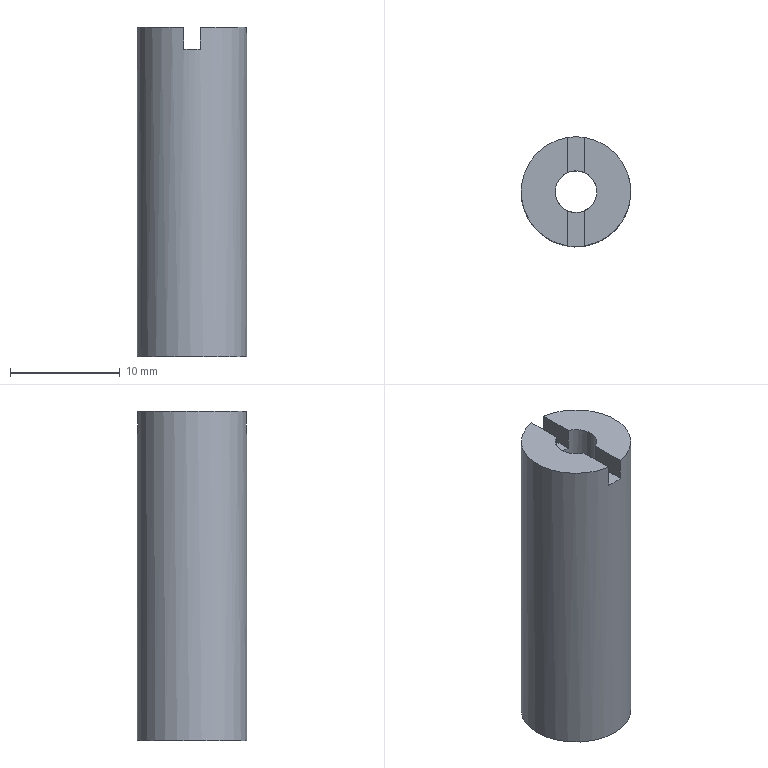Part | NX | features solid 2 | 1 solid | 13 faces | box 10 x 10 x 30 mm | volume 1574 mm3 | plane 10 | cylinder 3 | commonest cylinder face diameters 3.8 x1 6 x1 10 x1
STEP:
#1=CARTESIAN_POINT('',(0.75,307.085,-13.));
#2=VERTEX_POINT('',#1);
#3=CARTESIAN_POINT('',(0.75,307.085,-11.));
#4=VERTEX_POINT('',#3);
#5=CARTESIAN_POINT('',(0.75,307.085,-41.));
#6=DIRECTION('',(0.,0.,1.));
#7=VECTOR('',#6,1000.);
#8=LINE('',#5,#7);
#9=EDGE_CURVE('',#2,#4,#8,.T.);
#10=ORIENTED_EDGE('',*,*,#9,.F.);
#11=CARTESIAN_POINT('',(-0.75,307.085,-13.));
#12=VERTEX_POINT('',#11);
#13=CARTESIAN_POINT('',(0.,312.028,-13.));
#14=DIRECTION('',(0.,0.,1.));
#15=DIRECTION('',(1.,0.,0.));
#16=AXIS2_PLACEMENT_3D('',#13,#14,#15);
#17=CIRCLE('',#16,5.);
#18=EDGE_CURVE('',#12,#2,#17,.T.);
#19=ORIENTED_EDGE('',*,*,#18,.F.);
#20=CARTESIAN_POINT('',(-0.75,307.085,-11.));
#21=VERTEX_POINT('',#20);
#22=CARTESIAN_POINT('',(-0.75,307.085,-41.));
#23=DIRECTION('',(0.,0.,1.));
#24=VECTOR('',#23,1000.);
#25=LINE('',#22,#24);
#26=EDGE_CURVE('',#12,#21,#25,.T.);
#27=ORIENTED_EDGE('',*,*,#26,.T.);
#28=CARTESIAN_POINT('',(-0.75,316.971,-11.));
#29=VERTEX_POINT('',#28);
#30=CARTESIAN_POINT('',(0.,312.028,-11.));
#31=DIRECTION('',(0.,0.,1.));
#32=DIRECTION('',(1.,0.,0.));
#33=AXIS2_PLACEMENT_3D('',#30,#31,#32);
#34=CIRCLE('',#33,5.);
#35=EDGE_CURVE('',#29,#21,#34,.T.);
#36=ORIENTED_EDGE('',*,*,#35,.F.);
#37=CARTESIAN_POINT('',(-0.75,316.971,-13.));
#38=VERTEX_POINT('',#37);
#39=CARTESIAN_POINT('',(-0.75,316.971,-41.));
#40=DIRECTION('',(0.,0.,-1.));
#41=VECTOR('',#40,1000.);
#42=LINE('',#39,#41);
#43=EDGE_CURVE('',#29,#38,#42,.T.);
#44=ORIENTED_EDGE('',*,*,#43,.T.);
#45=CARTESIAN_POINT('',(0.75,316.971,-13.));
#46=VERTEX_POINT('',#45);
#47=CARTESIAN_POINT('',(0.,312.028,-13.));
#48=DIRECTION('',(0.,0.,1.));
#49=DIRECTION('',(1.,0.,0.));
#50=AXIS2_PLACEMENT_3D('',#47,#48,#49);
#51=CIRCLE('',#50,5.);
#52=EDGE_CURVE('',#46,#38,#51,.T.);
#53=ORIENTED_EDGE('',*,*,#52,.F.);
#54=CARTESIAN_POINT('',(0.75,316.971,-11.));
#55=VERTEX_POINT('',#54);
#56=CARTESIAN_POINT('',(0.75,316.971,-41.));
#57=DIRECTION('',(0.,0.,-1.));
#58=VECTOR('',#57,1000.);
#59=LINE('',#56,#58);
#60=EDGE_CURVE('',#55,#46,#59,.T.);
#61=ORIENTED_EDGE('',*,*,#60,.F.);
#62=CARTESIAN_POINT('',(0.,312.028,-11.));
#63=DIRECTION('',(0.,0.,1.));
#64=DIRECTION('',(1.,0.,0.));
#65=AXIS2_PLACEMENT_3D('',#62,#63,#64);
#66=CIRCLE('',#65,5.);
#67=EDGE_CURVE('',#4,#55,#66,.T.);
#68=ORIENTED_EDGE('',*,*,#67,.F.);
#69=EDGE_LOOP('',(#10,#19,#27,#36,#44,#53,#61,#68));
#70=FACE_BOUND('',#69,.T.);
#71=CARTESIAN_POINT('',(5.,312.028,-41.));
#72=VERTEX_POINT('',#71);
#73=CARTESIAN_POINT('',(0.,312.028,-41.));
#74=DIRECTION('',(0.,0.,1.));
#75=DIRECTION('',(1.,0.,0.));
#76=AXIS2_PLACEMENT_3D('',#73,#74,#75);
#77=CIRCLE('',#76,5.);
#78=EDGE_CURVE('',#72,#72,#77,.T.);
#79=ORIENTED_EDGE('',*,*,#78,.T.);
#80=EDGE_LOOP('',(#79));
#81=FACE_BOUND('',#80,.T.);
#82=CARTESIAN_POINT('',(0.,312.028,-41.));
#83=DIRECTION('',(0.,0.,1.));
#84=DIRECTION('',(-1.,0.,0.));
#85=AXIS2_PLACEMENT_3D('',#82,#83,#84);
#86=CYLINDRICAL_SURFACE('',#85,5.);
#87=ADVANCED_FACE('',(#70,#81),#86,.T.);
#88=ORIENTED_EDGE('',*,*,#35,.T.);
#89=CARTESIAN_POINT('',(-0.75,310.282,-11.));
#90=VERTEX_POINT('',#89);
#91=CARTESIAN_POINT('',(-0.75,317.028,-11.));
#92=DIRECTION('',(0.,-1.,0.));
#93=VECTOR('',#92,1000.);
#94=LINE('',#91,#93);
#95=EDGE_CURVE('',#90,#21,#94,.T.);
#96=ORIENTED_EDGE('',*,*,#95,.F.);
#97=CARTESIAN_POINT('',(-0.75,313.774,-11.));
#98=VERTEX_POINT('',#97);
#99=CARTESIAN_POINT('',(0.,312.028,-11.));
#100=DIRECTION('',(0.,0.,1.));
#101=DIRECTION('',(1.,0.,0.));
#102=AXIS2_PLACEMENT_3D('',#99,#100,#101);
#103=CIRCLE('',#102,1.9);
#104=EDGE_CURVE('',#98,#90,#103,.T.);
#105=ORIENTED_EDGE('',*,*,#104,.F.);
#106=CARTESIAN_POINT('',(-0.75,317.028,-11.));
#107=DIRECTION('',(0.,-1.,0.));
#108=VECTOR('',#107,1000.);
#109=LINE('',#106,#108);
#110=EDGE_CURVE('',#29,#98,#109,.T.);
#111=ORIENTED_EDGE('',*,*,#110,.F.);
#112=EDGE_LOOP('',(#88,#96,#105,#111));
#113=FACE_BOUND('',#112,.T.);
#114=CARTESIAN_POINT('',(0.,312.028,-11.));
#115=DIRECTION('',(0.,0.,1.));
#116=DIRECTION('',(-1.,0.,0.));
#117=AXIS2_PLACEMENT_3D('',#114,#115,#116);
#118=PLANE('',#117);
#119=ADVANCED_FACE('',(#113),#118,.T.);
#120=CARTESIAN_POINT('',(3.,312.028,-41.));
#121=VERTEX_POINT('',#120);
#122=CARTESIAN_POINT('',(0.,312.028,-41.));
#123=DIRECTION('',(0.,0.,1.));
#124=DIRECTION('',(1.,0.,0.));
#125=AXIS2_PLACEMENT_3D('',#122,#123,#124);
#126=CIRCLE('',#125,3.);
#127=EDGE_CURVE('',#121,#121,#126,.T.);
#128=ORIENTED_EDGE('',*,*,#127,.T.);
#129=EDGE_LOOP('',(#128));
#130=FACE_BOUND('',#129,.T.);
#131=ORIENTED_EDGE('',*,*,#78,.F.);
#132=EDGE_LOOP('',(#131));
#133=FACE_BOUND('',#132,.T.);
#134=CARTESIAN_POINT('',(0.,312.028,-41.));
#135=DIRECTION('',(0.,0.,1.));
#136=DIRECTION('',(-1.,0.,0.));
#137=AXIS2_PLACEMENT_3D('',#134,#135,#136);
#138=PLANE('',#137);
#139=ADVANCED_FACE('',(#130,#133),#138,.F.);
#140=CARTESIAN_POINT('',(0.75,310.282,-11.));
#141=VERTEX_POINT('',#140);
#142=CARTESIAN_POINT('',(0.75,317.028,-11.));
#143=DIRECTION('',(0.,-1.,0.));
#144=VECTOR('',#143,1000.);
#145=LINE('',#142,#144);
#146=EDGE_CURVE('',#141,#4,#145,.T.);
#147=ORIENTED_EDGE('',*,*,#146,.T.);
#148=ORIENTED_EDGE('',*,*,#67,.T.);
#149=CARTESIAN_POINT('',(0.75,313.774,-11.));
#150=VERTEX_POINT('',#149);
#151=CARTESIAN_POINT('',(0.75,317.028,-11.));
#152=DIRECTION('',(0.,-1.,0.));
#153=VECTOR('',#152,1000.);
#154=LINE('',#151,#153);
#155=EDGE_CURVE('',#55,#150,#154,.T.);
#156=ORIENTED_EDGE('',*,*,#155,.T.);
#157=CARTESIAN_POINT('',(0.,312.028,-11.));
#158=DIRECTION('',(0.,0.,1.));
#159=DIRECTION('',(1.,0.,0.));
#160=AXIS2_PLACEMENT_3D('',#157,#158,#159);
#161=CIRCLE('',#160,1.9);
#162=EDGE_CURVE('',#141,#150,#161,.T.);
#163=ORIENTED_EDGE('',*,*,#162,.F.);
#164=EDGE_LOOP('',(#147,#148,#156,#163));
#165=FACE_BOUND('',#164,.T.);
#166=CARTESIAN_POINT('',(0.,312.028,-11.));
#167=DIRECTION('',(0.,0.,1.));
#168=DIRECTION('',(-1.,0.,0.));
#169=AXIS2_PLACEMENT_3D('',#166,#167,#168);
#170=PLANE('',#169);
#171=ADVANCED_FACE('',(#165),#170,.T.);
#172=CARTESIAN_POINT('',(1.9,312.028,-16.));
#173=VERTEX_POINT('',#172);
#174=CARTESIAN_POINT('',(0.,312.028,-16.));
#175=DIRECTION('',(0.,0.,-1.));
#176=DIRECTION('',(1.,0.,0.));
#177=AXIS2_PLACEMENT_3D('',#174,#175,#176);
#178=CIRCLE('',#177,1.9);
#179=EDGE_CURVE('',#173,#173,#178,.T.);
#180=ORIENTED_EDGE('',*,*,#179,.T.);
#181=EDGE_LOOP('',(#180));
#182=FACE_BOUND('',#181,.T.);
#183=ORIENTED_EDGE('',*,*,#162,.T.);
#184=CARTESIAN_POINT('',(0.75,313.774,-13.));
#185=VERTEX_POINT('',#184);
#186=CARTESIAN_POINT('',(0.75,313.774,-16.));
#187=DIRECTION('',(0.,0.,-1.));
#188=VECTOR('',#187,1000.);
#189=LINE('',#186,#188);
#190=EDGE_CURVE('',#150,#185,#189,.T.);
#191=ORIENTED_EDGE('',*,*,#190,.T.);
#192=CARTESIAN_POINT('',(-0.75,313.774,-13.));
#193=VERTEX_POINT('',#192);
#194=CARTESIAN_POINT('',(0.,312.028,-13.));
#195=DIRECTION('',(0.,0.,1.));
#196=DIRECTION('',(1.,0.,0.));
#197=AXIS2_PLACEMENT_3D('',#194,#195,#196);
#198=CIRCLE('',#197,1.9);
#199=EDGE_CURVE('',#185,#193,#198,.T.);
#200=ORIENTED_EDGE('',*,*,#199,.T.);
#201=CARTESIAN_POINT('',(-0.75,313.774,-16.));
#202=DIRECTION('',(0.,0.,-1.));
#203=VECTOR('',#202,1000.);
#204=LINE('',#201,#203);
#205=EDGE_CURVE('',#98,#193,#204,.T.);
#206=ORIENTED_EDGE('',*,*,#205,.F.);
#207=ORIENTED_EDGE('',*,*,#104,.T.);
#208=CARTESIAN_POINT('',(-0.75,310.282,-13.));
#209=VERTEX_POINT('',#208);
#210=CARTESIAN_POINT('',(-0.75,310.282,-16.));
#211=DIRECTION('',(0.,0.,1.));
#212=VECTOR('',#211,1000.);
#213=LINE('',#210,#212);
#214=EDGE_CURVE('',#209,#90,#213,.T.);
#215=ORIENTED_EDGE('',*,*,#214,.F.);
#216=CARTESIAN_POINT('',(0.75,310.282,-13.));
#217=VERTEX_POINT('',#216);
#218=CARTESIAN_POINT('',(0.,312.028,-13.));
#219=DIRECTION('',(0.,0.,1.));
#220=DIRECTION('',(1.,0.,0.));
#221=AXIS2_PLACEMENT_3D('',#218,#219,#220);
#222=CIRCLE('',#221,1.9);
#223=EDGE_CURVE('',#209,#217,#222,.T.);
#224=ORIENTED_EDGE('',*,*,#223,.T.);
#225=CARTESIAN_POINT('',(0.75,310.282,-16.));
#226=DIRECTION('',(0.,0.,1.));
#227=VECTOR('',#226,1000.);
#228=LINE('',#225,#227);
#229=EDGE_CURVE('',#217,#141,#228,.T.);
#230=ORIENTED_EDGE('',*,*,#229,.T.);
#231=EDGE_LOOP('',(#183,#191,#200,#206,#207,#215,#224,#230));
#232=FACE_BOUND('',#231,.T.);
#233=CARTESIAN_POINT('',(0.,312.028,-16.));
#234=DIRECTION('',(0.,0.,1.));
#235=DIRECTION('',(-1.,0.,0.));
#236=AXIS2_PLACEMENT_3D('',#233,#234,#235);
#237=CYLINDRICAL_SURFACE('',#236,1.9);
#238=ADVANCED_FACE('',(#182,#232),#237,.F.);
#239=CARTESIAN_POINT('',(3.,312.028,-16.));
#240=VERTEX_POINT('',#239);
#241=CARTESIAN_POINT('',(0.,312.028,-16.));
#242=DIRECTION('',(0.,0.,1.));
#243=DIRECTION('',(1.,0.,0.));
#244=AXIS2_PLACEMENT_3D('',#241,#242,#243);
#245=CIRCLE('',#244,3.);
#246=EDGE_CURVE('',#240,#240,#245,.T.);
#247=ORIENTED_EDGE('',*,*,#246,.F.);
#248=EDGE_LOOP('',(#247));
#249=FACE_BOUND('',#248,.T.);
#250=ORIENTED_EDGE('',*,*,#179,.F.);
#251=EDGE_LOOP('',(#250));
#252=FACE_BOUND('',#251,.T.);
#253=CARTESIAN_POINT('',(0.,312.028,-16.));
#254=DIRECTION('',(0.,0.,1.));
#255=DIRECTION('',(-1.,0.,0.));
#256=AXIS2_PLACEMENT_3D('',#253,#254,#255);
#257=PLANE('',#256);
#258=ADVANCED_FACE('',(#249,#252),#257,.F.);
#259=ORIENTED_EDGE('',*,*,#127,.F.);
#260=EDGE_LOOP('',(#259));
#261=FACE_BOUND('',#260,.T.);
#262=ORIENTED_EDGE('',*,*,#246,.T.);
#263=EDGE_LOOP('',(#262));
#264=FACE_BOUND('',#263,.T.);
#265=CARTESIAN_POINT('',(0.,312.028,-41.));
#266=DIRECTION('',(0.,0.,1.));
#267=DIRECTION('',(-1.,0.,0.));
#268=AXIS2_PLACEMENT_3D('',#265,#266,#267);
#269=CYLINDRICAL_SURFACE('',#268,3.);
#270=ADVANCED_FACE('',(#261,#264),#269,.F.);
#271=ORIENTED_EDGE('',*,*,#9,.T.);
#272=ORIENTED_EDGE('',*,*,#146,.F.);
#273=ORIENTED_EDGE('',*,*,#229,.F.);
#274=CARTESIAN_POINT('',(0.75,317.028,-13.));
#275=DIRECTION('',(0.,-1.,0.));
#276=VECTOR('',#275,1000.);
#277=LINE('',#274,#276);
#278=EDGE_CURVE('',#217,#2,#277,.T.);
#279=ORIENTED_EDGE('',*,*,#278,.T.);
#280=EDGE_LOOP('',(#271,#272,#273,#279));
#281=FACE_BOUND('',#280,.T.);
#282=CARTESIAN_POINT('',(0.75,317.028,-11.));
#283=DIRECTION('',(1.,0.,0.));
#284=DIRECTION('',(0.,0.,1.));
#285=AXIS2_PLACEMENT_3D('',#282,#283,#284);
#286=PLANE('',#285);
#287=ADVANCED_FACE('',(#281),#286,.F.);
#288=CARTESIAN_POINT('',(-0.75,317.028,-13.));
#289=DIRECTION('',(0.,-1.,0.));
#290=VECTOR('',#289,1000.);
#291=LINE('',#288,#290);
#292=EDGE_CURVE('',#209,#12,#291,.T.);
#293=ORIENTED_EDGE('',*,*,#292,.F.);
#294=ORIENTED_EDGE('',*,*,#214,.T.);
#295=ORIENTED_EDGE('',*,*,#95,.T.);
#296=ORIENTED_EDGE('',*,*,#26,.F.);
#297=EDGE_LOOP('',(#293,#294,#295,#296));
#298=FACE_BOUND('',#297,.T.);
#299=CARTESIAN_POINT('',(-0.75,317.028,-11.));
#300=DIRECTION('',(1.,0.,0.));
#301=DIRECTION('',(0.,0.,1.));
#302=AXIS2_PLACEMENT_3D('',#299,#300,#301);
#303=PLANE('',#302);
#304=ADVANCED_FACE('',(#298),#303,.T.);
#305=ORIENTED_EDGE('',*,*,#18,.T.);
#306=ORIENTED_EDGE('',*,*,#278,.F.);
#307=ORIENTED_EDGE('',*,*,#223,.F.);
#308=ORIENTED_EDGE('',*,*,#292,.T.);
#309=EDGE_LOOP('',(#305,#306,#307,#308));
#310=FACE_BOUND('',#309,.T.);
#311=CARTESIAN_POINT('',(0.,317.028,-13.));
#312=DIRECTION('',(0.,0.,1.));
#313=DIRECTION('',(0.,1.,0.));
#314=AXIS2_PLACEMENT_3D('',#311,#312,#313);
#315=PLANE('',#314);
#316=ADVANCED_FACE('',(#310),#315,.T.);
#317=ORIENTED_EDGE('',*,*,#52,.T.);
#318=CARTESIAN_POINT('',(-0.75,317.028,-13.));
#319=DIRECTION('',(0.,-1.,0.));
#320=VECTOR('',#319,1000.);
#321=LINE('',#318,#320);
#322=EDGE_CURVE('',#38,#193,#321,.T.);
#323=ORIENTED_EDGE('',*,*,#322,.T.);
#324=ORIENTED_EDGE('',*,*,#199,.F.);
#325=CARTESIAN_POINT('',(0.75,317.028,-13.));
#326=DIRECTION('',(0.,-1.,0.));
#327=VECTOR('',#326,1000.);
#328=LINE('',#325,#327);
#329=EDGE_CURVE('',#46,#185,#328,.T.);
#330=ORIENTED_EDGE('',*,*,#329,.F.);
#331=EDGE_LOOP('',(#317,#323,#324,#330));
#332=FACE_BOUND('',#331,.T.);
#333=CARTESIAN_POINT('',(0.,317.028,-13.));
#334=DIRECTION('',(0.,0.,1.));
#335=DIRECTION('',(0.,1.,0.));
#336=AXIS2_PLACEMENT_3D('',#333,#334,#335);
#337=PLANE('',#336);
#338=ADVANCED_FACE('',(#332),#337,.T.);
#339=ORIENTED_EDGE('',*,*,#60,.T.);
#340=ORIENTED_EDGE('',*,*,#329,.T.);
#341=ORIENTED_EDGE('',*,*,#190,.F.);
#342=ORIENTED_EDGE('',*,*,#155,.F.);
#343=EDGE_LOOP('',(#339,#340,#341,#342));
#344=FACE_BOUND('',#343,.T.);
#345=CARTESIAN_POINT('',(0.75,317.028,-11.));
#346=DIRECTION('',(1.,0.,0.));
#347=DIRECTION('',(0.,0.,1.));
#348=AXIS2_PLACEMENT_3D('',#345,#346,#347);
#349=PLANE('',#348);
#350=ADVANCED_FACE('',(#344),#349,.F.);
#351=ORIENTED_EDGE('',*,*,#110,.T.);
#352=ORIENTED_EDGE('',*,*,#205,.T.);
#353=ORIENTED_EDGE('',*,*,#322,.F.);
#354=ORIENTED_EDGE('',*,*,#43,.F.);
#355=EDGE_LOOP('',(#351,#352,#353,#354));
#356=FACE_BOUND('',#355,.T.);
#357=CARTESIAN_POINT('',(-0.75,317.028,-11.));
#358=DIRECTION('',(1.,0.,0.));
#359=DIRECTION('',(0.,0.,1.));
#360=AXIS2_PLACEMENT_3D('',#357,#358,#359);
#361=PLANE('',#360);
#362=ADVANCED_FACE('',(#356),#361,.T.);
#363=CLOSED_SHELL('',(#87,#119,#139,#171,#238,#258,#270,#287,#304,#316,#338,#350,#362));
#364=MANIFOLD_SOLID_BREP('',#363);
#365=(LENGTH_UNIT()NAMED_UNIT(*)SI_UNIT(.MILLI.,.METRE.));
#366=UNCERTAINTY_MEASURE_WITH_UNIT(LENGTH_MEASURE(0.00001),#365,'','');
#367=(NAMED_UNIT(*)PLANE_ANGLE_UNIT()SI_UNIT($,.RADIAN.));
#368=(NAMED_UNIT(*)SI_UNIT($,.STERADIAN.)SOLID_ANGLE_UNIT());
#369=(GEOMETRIC_REPRESENTATION_CONTEXT(3)GLOBAL_UNCERTAINTY_ASSIGNED_CONTEXT((#366))GLOBAL_UNIT_ASSIGNED_CONTEXT((#365,#367,#368))REPRESENTATION_CONTEXT('',''));
#370=ADVANCED_BREP_SHAPE_REPRESENTATION('',(#364),#369);